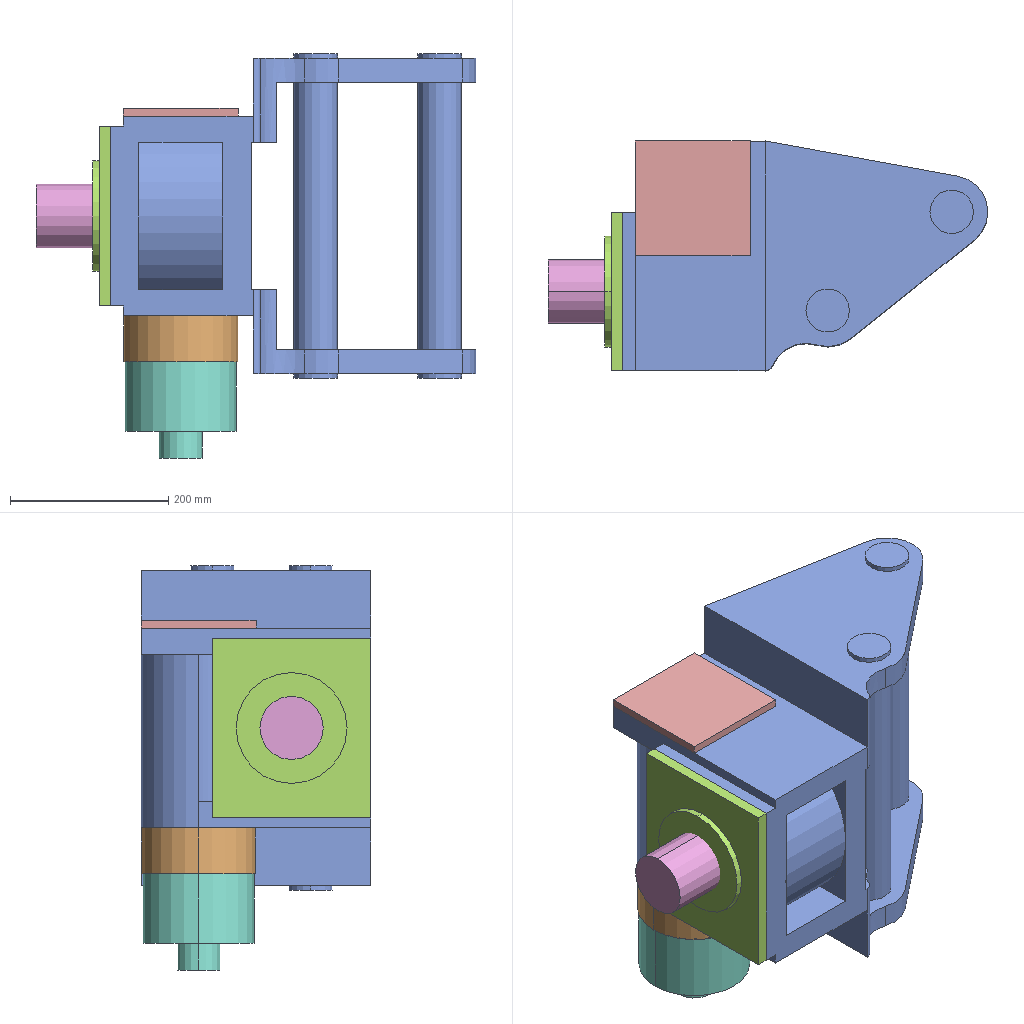Assembly | SolidWorks | 6 different items | 6 placed | box 555 x 290 x 511 mm
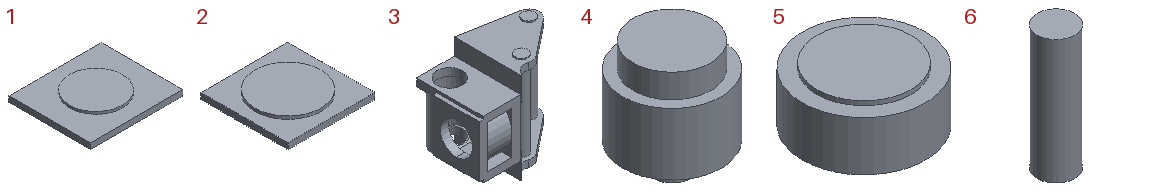Parts list (item | quantity | size | volume | features):
1 | x1 | 227 x 200 x 28 mm | 838390 mm3 | features ICE 2, Extrusion 1
2 | x1 | 145 x 145 x 15 mm | 257767 mm3 | features Extrusion 1, ICE 1
3 | x1 | 461.6 x 289.885 x 410 mm | 11100203 mm3 | features ICE 17, Extrusion 1, MirrorPattern 1
4 | x1 | 140 x 140 x 156 mm | 1755635 mm3 | features ICE 2, Extrusion 1
5 | x1 | 144 x 144 x 63 mm | 992106 mm3 | features Extrusion 1, ICE 1
6 | x1 | 80 x 80 x 263.5 mm | 1324495 mm3 | features Extrusion 1
Mates (type | each side: item.copy, entity, surface, feature):
Concentric | 4.1 face cylinder Boss-Extrude2 | 5.1 face cylinder Boss-Extrude1
Coincident | 4.1 face plane Boss-Extrude2 | 5.1 face plane Boss-Extrude1
Concentric | 3.1 face cylinder Cut-Extrude3 | 5.1 face cylinder Boss-Extrude1
Coincident | 3.1 face plane Boss-Extrude1 | 5.1 face plane Boss-Extrude1
Concentric | 2.1 face cylinder Boss-Extrude2 | 3.1 face cylinder Cut-Extrude2
Coincident | 2.1 face plane Boss-Extrude1 | 3.1 face plane Boss-Extrude1
Coincident | 2.1 face plane Boss-Extrude1 | 3.1 face plane Boss-Extrude2
Concentric | 3.1 face cylinder Cut-Extrude4 | 6.1 face cylinder Boss-Extrude1
Coincident | 3.1 face plane Cut-Extrude5 | 6.1 face plane Boss-Extrude1
Coincident | 3.1 face plane Boss-Extrude5 | 1.1 face plane Boss-Extrude1
Concentric | 3.1 face cylinder Cut-Extrude4 | 1.1 face cylinder Boss-Extrude2